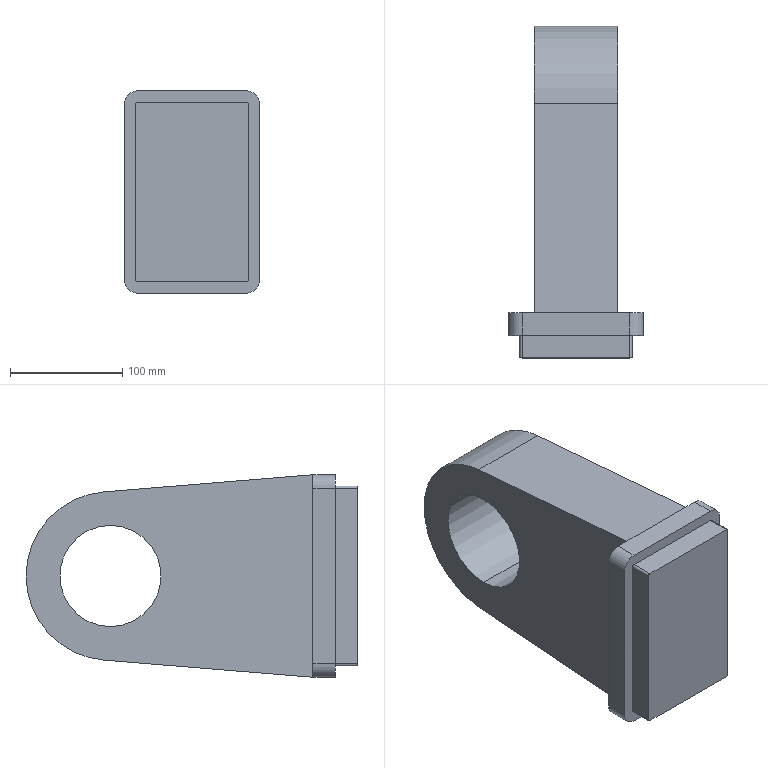Part | SolidWorks | features ICE 2, Extrusion 1 | 1 solid | 27 faces | box 120 x 295 x 180 mm | volume 3133759 mm3 | plane 16 | cylinder 11 | commonest cylinder face diameters 4 x4 24 x4 90 x2 150 x1
STEP:
#1=CARTESIAN_POINT('',(37.,200.,45.));
#2=VERTEX_POINT('',#1);
#3=CARTESIAN_POINT('',(37.,200.,-45.));
#4=VERTEX_POINT('',#3);
#5=CARTESIAN_POINT('',(37.,200.,0.));
#6=DIRECTION('',(1.,0.,0.));
#7=DIRECTION('',(0.,0.,-1.));
#8=AXIS2_PLACEMENT_3D('',#5,#6,#7);
#9=CIRCLE('',#8,45.);
#10=EDGE_CURVE('',#2,#4,#9,.T.);
#11=ORIENTED_EDGE('',*,*,#10,.T.);
#12=CARTESIAN_POINT('',(-37.,200.,-45.));
#13=VERTEX_POINT('',#12);
#14=CARTESIAN_POINT('',(37.,200.,-45.));
#15=DIRECTION('',(-1.,0.,0.));
#16=VECTOR('',#15,1000.);
#17=LINE('',#14,#16);
#18=EDGE_CURVE('',#4,#13,#17,.T.);
#19=ORIENTED_EDGE('',*,*,#18,.T.);
#20=CARTESIAN_POINT('',(-37.,200.,45.));
#21=VERTEX_POINT('',#20);
#22=CARTESIAN_POINT('',(-37.,200.,0.));
#23=DIRECTION('',(1.,0.,0.));
#24=DIRECTION('',(0.,0.,-1.));
#25=AXIS2_PLACEMENT_3D('',#22,#23,#24);
#26=CIRCLE('',#25,45.);
#27=EDGE_CURVE('',#21,#13,#26,.T.);
#28=ORIENTED_EDGE('',*,*,#27,.F.);
#29=CARTESIAN_POINT('',(37.,200.,45.));
#30=DIRECTION('',(-1.,0.,0.));
#31=VECTOR('',#30,1000.);
#32=LINE('',#29,#31);
#33=EDGE_CURVE('',#2,#21,#32,.T.);
#34=ORIENTED_EDGE('',*,*,#33,.F.);
#35=EDGE_LOOP('',(#11,#19,#28,#34));
#36=FACE_OUTER_BOUND('',#35,.T.);
#37=CARTESIAN_POINT('',(37.,200.,0.));
#38=DIRECTION('',(-1.,0.,0.));
#39=DIRECTION('',(0.,0.,1.));
#40=AXIS2_PLACEMENT_3D('',#37,#38,#39);
#41=CYLINDRICAL_SURFACE('',#40,45.);
#42=ADVANCED_FACE('',(#36),#41,.F.);
#43=CARTESIAN_POINT('',(-48.,20.,90.));
#44=VERTEX_POINT('',#43);
#45=CARTESIAN_POINT('',(-37.,20.,90.));
#46=VERTEX_POINT('',#45);
#47=CARTESIAN_POINT('',(48.,20.,90.));
#48=DIRECTION('',(1.,0.,0.));
#49=VECTOR('',#48,1000.);
#50=LINE('',#47,#49);
#51=EDGE_CURVE('',#44,#46,#50,.T.);
#52=ORIENTED_EDGE('',*,*,#51,.T.);
#53=CARTESIAN_POINT('',(-37.,20.,-90.));
#54=VERTEX_POINT('',#53);
#55=CARTESIAN_POINT('',(-37.,20.,90.));
#56=DIRECTION('',(0.,0.,-1.));
#57=VECTOR('',#56,1000.);
#58=LINE('',#55,#57);
#59=EDGE_CURVE('',#46,#54,#58,.T.);
#60=ORIENTED_EDGE('',*,*,#59,.T.);
#61=CARTESIAN_POINT('',(-48.,20.,-90.));
#62=VERTEX_POINT('',#61);
#63=CARTESIAN_POINT('',(48.,20.,-90.));
#64=DIRECTION('',(-1.,0.,0.));
#65=VECTOR('',#64,1000.);
#66=LINE('',#63,#65);
#67=EDGE_CURVE('',#54,#62,#66,.T.);
#68=ORIENTED_EDGE('',*,*,#67,.T.);
#69=CARTESIAN_POINT('',(-60.,20.,-78.));
#70=VERTEX_POINT('',#69);
#71=CARTESIAN_POINT('',(-48.,20.,-78.));
#72=DIRECTION('',(0.,1.,0.));
#73=DIRECTION('',(0.,0.,1.));
#74=AXIS2_PLACEMENT_3D('',#71,#72,#73);
#75=CIRCLE('',#74,12.);
#76=EDGE_CURVE('',#62,#70,#75,.T.);
#77=ORIENTED_EDGE('',*,*,#76,.T.);
#78=CARTESIAN_POINT('',(-60.,20.,78.));
#79=VERTEX_POINT('',#78);
#80=CARTESIAN_POINT('',(-60.,20.,-78.));
#81=DIRECTION('',(0.,0.,1.));
#82=VECTOR('',#81,1000.);
#83=LINE('',#80,#82);
#84=EDGE_CURVE('',#70,#79,#83,.T.);
#85=ORIENTED_EDGE('',*,*,#84,.T.);
#86=CARTESIAN_POINT('',(-48.,20.,78.));
#87=DIRECTION('',(0.,1.,0.));
#88=DIRECTION('',(0.,0.,-1.));
#89=AXIS2_PLACEMENT_3D('',#86,#87,#88);
#90=CIRCLE('',#89,12.);
#91=EDGE_CURVE('',#79,#44,#90,.T.);
#92=ORIENTED_EDGE('',*,*,#91,.T.);
#93=EDGE_LOOP('',(#52,#60,#68,#77,#85,#92));
#94=FACE_OUTER_BOUND('',#93,.T.);
#95=CARTESIAN_POINT('',(-48.,20.,-78.));
#96=DIRECTION('',(0.,1.,0.));
#97=DIRECTION('',(0.,0.,1.));
#98=AXIS2_PLACEMENT_3D('',#95,#96,#97);
#99=PLANE('',#98);
#100=ADVANCED_FACE('',(#94),#99,.T.);
#101=CARTESIAN_POINT('',(-48.,0.,-90.));
#102=VERTEX_POINT('',#101);
#103=CARTESIAN_POINT('',(-60.,0.,-78.));
#104=VERTEX_POINT('',#103);
#105=CARTESIAN_POINT('',(-48.,0.,-78.));
#106=DIRECTION('',(0.,1.,0.));
#107=DIRECTION('',(0.,0.,1.));
#108=AXIS2_PLACEMENT_3D('',#105,#106,#107);
#109=CIRCLE('',#108,12.);
#110=EDGE_CURVE('',#102,#104,#109,.T.);
#111=ORIENTED_EDGE('',*,*,#110,.F.);
#112=CARTESIAN_POINT('',(48.,0.,-90.));
#113=VERTEX_POINT('',#112);
#114=CARTESIAN_POINT('',(48.,0.,-90.));
#115=DIRECTION('',(-1.,0.,0.));
#116=VECTOR('',#115,1000.);
#117=LINE('',#114,#116);
#118=EDGE_CURVE('',#113,#102,#117,.T.);
#119=ORIENTED_EDGE('',*,*,#118,.F.);
#120=CARTESIAN_POINT('',(60.,0.,-78.));
#121=VERTEX_POINT('',#120);
#122=CARTESIAN_POINT('',(48.,0.,-78.));
#123=DIRECTION('',(0.,1.,0.));
#124=DIRECTION('',(0.,0.,-1.));
#125=AXIS2_PLACEMENT_3D('',#122,#123,#124);
#126=CIRCLE('',#125,12.);
#127=EDGE_CURVE('',#121,#113,#126,.T.);
#128=ORIENTED_EDGE('',*,*,#127,.F.);
#129=CARTESIAN_POINT('',(60.,0.,78.));
#130=VERTEX_POINT('',#129);
#131=CARTESIAN_POINT('',(60.,0.,-78.));
#132=DIRECTION('',(0.,0.,-1.));
#133=VECTOR('',#132,1000.);
#134=LINE('',#131,#133);
#135=EDGE_CURVE('',#130,#121,#134,.T.);
#136=ORIENTED_EDGE('',*,*,#135,.F.);
#137=CARTESIAN_POINT('',(48.,0.,90.));
#138=VERTEX_POINT('',#137);
#139=CARTESIAN_POINT('',(48.,0.,78.));
#140=DIRECTION('',(0.,1.,0.));
#141=DIRECTION('',(0.,0.,1.));
#142=AXIS2_PLACEMENT_3D('',#139,#140,#141);
#143=CIRCLE('',#142,12.);
#144=EDGE_CURVE('',#138,#130,#143,.T.);
#145=ORIENTED_EDGE('',*,*,#144,.F.);
#146=CARTESIAN_POINT('',(-48.,0.,90.));
#147=VERTEX_POINT('',#146);
#148=CARTESIAN_POINT('',(48.,0.,90.));
#149=DIRECTION('',(1.,0.,0.));
#150=VECTOR('',#149,1000.);
#151=LINE('',#148,#150);
#152=EDGE_CURVE('',#147,#138,#151,.T.);
#153=ORIENTED_EDGE('',*,*,#152,.F.);
#154=CARTESIAN_POINT('',(-60.,0.,78.));
#155=VERTEX_POINT('',#154);
#156=CARTESIAN_POINT('',(-48.,0.,78.));
#157=DIRECTION('',(0.,1.,0.));
#158=DIRECTION('',(0.,0.,-1.));
#159=AXIS2_PLACEMENT_3D('',#156,#157,#158);
#160=CIRCLE('',#159,12.);
#161=EDGE_CURVE('',#155,#147,#160,.T.);
#162=ORIENTED_EDGE('',*,*,#161,.F.);
#163=CARTESIAN_POINT('',(-60.,0.,-78.));
#164=DIRECTION('',(0.,0.,1.));
#165=VECTOR('',#164,1000.);
#166=LINE('',#163,#165);
#167=EDGE_CURVE('',#104,#155,#166,.T.);
#168=ORIENTED_EDGE('',*,*,#167,.F.);
#169=EDGE_LOOP('',(#111,#119,#128,#136,#145,#153,#162,#168));
#170=FACE_OUTER_BOUND('',#169,.T.);
#171=CARTESIAN_POINT('',(-50.,0.,-78.));
#172=VERTEX_POINT('',#171);
#173=CARTESIAN_POINT('',(-48.,0.,-80.));
#174=VERTEX_POINT('',#173);
#175=CARTESIAN_POINT('',(-48.,0.,-78.));
#176=DIRECTION('',(0.,-1.,0.));
#177=DIRECTION('',(0.,0.,-1.));
#178=AXIS2_PLACEMENT_3D('',#175,#176,#177);
#179=CIRCLE('',#178,2.);
#180=EDGE_CURVE('',#172,#174,#179,.T.);
#181=ORIENTED_EDGE('',*,*,#180,.F.);
#182=CARTESIAN_POINT('',(-50.,0.,78.));
#183=VERTEX_POINT('',#182);
#184=CARTESIAN_POINT('',(-50.,0.,78.));
#185=DIRECTION('',(0.,0.,-1.));
#186=VECTOR('',#185,1000.);
#187=LINE('',#184,#186);
#188=EDGE_CURVE('',#183,#172,#187,.T.);
#189=ORIENTED_EDGE('',*,*,#188,.F.);
#190=CARTESIAN_POINT('',(-48.,0.,80.));
#191=VERTEX_POINT('',#190);
#192=CARTESIAN_POINT('',(-48.,0.,78.));
#193=DIRECTION('',(0.,-1.,0.));
#194=DIRECTION('',(0.,0.,-1.));
#195=AXIS2_PLACEMENT_3D('',#192,#193,#194);
#196=CIRCLE('',#195,2.);
#197=EDGE_CURVE('',#191,#183,#196,.T.);
#198=ORIENTED_EDGE('',*,*,#197,.F.);
#199=CARTESIAN_POINT('',(48.,0.,80.));
#200=VERTEX_POINT('',#199);
#201=CARTESIAN_POINT('',(48.,0.,80.));
#202=DIRECTION('',(-1.,0.,0.));
#203=VECTOR('',#202,1000.);
#204=LINE('',#201,#203);
#205=EDGE_CURVE('',#200,#191,#204,.T.);
#206=ORIENTED_EDGE('',*,*,#205,.F.);
#207=CARTESIAN_POINT('',(50.,0.,78.));
#208=VERTEX_POINT('',#207);
#209=CARTESIAN_POINT('',(48.,0.,78.));
#210=DIRECTION('',(0.,-1.,0.));
#211=DIRECTION('',(0.,0.,-1.));
#212=AXIS2_PLACEMENT_3D('',#209,#210,#211);
#213=CIRCLE('',#212,2.);
#214=EDGE_CURVE('',#208,#200,#213,.T.);
#215=ORIENTED_EDGE('',*,*,#214,.F.);
#216=CARTESIAN_POINT('',(50.,0.,-78.));
#217=VERTEX_POINT('',#216);
#218=CARTESIAN_POINT('',(50.,0.,-78.));
#219=DIRECTION('',(0.,0.,1.));
#220=VECTOR('',#219,1000.);
#221=LINE('',#218,#220);
#222=EDGE_CURVE('',#217,#208,#221,.T.);
#223=ORIENTED_EDGE('',*,*,#222,.F.);
#224=CARTESIAN_POINT('',(48.,0.,-80.));
#225=VERTEX_POINT('',#224);
#226=CARTESIAN_POINT('',(48.,0.,-78.));
#227=DIRECTION('',(0.,-1.,0.));
#228=DIRECTION('',(0.,0.,-1.));
#229=AXIS2_PLACEMENT_3D('',#226,#227,#228);
#230=CIRCLE('',#229,2.);
#231=EDGE_CURVE('',#225,#217,#230,.T.);
#232=ORIENTED_EDGE('',*,*,#231,.F.);
#233=CARTESIAN_POINT('',(-48.,0.,-80.));
#234=DIRECTION('',(1.,0.,0.));
#235=VECTOR('',#234,1000.);
#236=LINE('',#233,#235);
#237=EDGE_CURVE('',#174,#225,#236,.T.);
#238=ORIENTED_EDGE('',*,*,#237,.F.);
#239=EDGE_LOOP('',(#181,#189,#198,#206,#215,#223,#232,#238));
#240=FACE_BOUND('',#239,.T.);
#241=CARTESIAN_POINT('',(-48.,0.,-78.));
#242=DIRECTION('',(0.,1.,0.));
#243=DIRECTION('',(0.,0.,1.));
#244=AXIS2_PLACEMENT_3D('',#241,#242,#243);
#245=PLANE('',#244);
#246=ADVANCED_FACE('',(#170,#240),#245,.F.);
#247=ORIENTED_EDGE('',*,*,#110,.T.);
#248=CARTESIAN_POINT('',(-60.,20.,-78.));
#249=DIRECTION('',(0.,-1.,0.));
#250=VECTOR('',#249,1000.);
#251=LINE('',#248,#250);
#252=EDGE_CURVE('',#70,#104,#251,.T.);
#253=ORIENTED_EDGE('',*,*,#252,.F.);
#254=ORIENTED_EDGE('',*,*,#76,.F.);
#255=CARTESIAN_POINT('',(-48.,20.,-90.));
#256=DIRECTION('',(0.,-1.,0.));
#257=VECTOR('',#256,1000.);
#258=LINE('',#255,#257);
#259=EDGE_CURVE('',#62,#102,#258,.T.);
#260=ORIENTED_EDGE('',*,*,#259,.T.);
#261=EDGE_LOOP('',(#247,#253,#254,#260));
#262=FACE_OUTER_BOUND('',#261,.T.);
#263=CARTESIAN_POINT('',(-48.,20.,-78.));
#264=DIRECTION('',(0.,-1.,0.));
#265=DIRECTION('',(0.,0.,-1.));
#266=AXIS2_PLACEMENT_3D('',#263,#264,#265);
#267=CYLINDRICAL_SURFACE('',#266,12.);
#268=ADVANCED_FACE('',(#262),#267,.T.);
#269=ORIENTED_EDGE('',*,*,#167,.T.);
#270=CARTESIAN_POINT('',(-60.,20.,78.));
#271=DIRECTION('',(0.,-1.,0.));
#272=VECTOR('',#271,1000.);
#273=LINE('',#270,#272);
#274=EDGE_CURVE('',#79,#155,#273,.T.);
#275=ORIENTED_EDGE('',*,*,#274,.F.);
#276=ORIENTED_EDGE('',*,*,#84,.F.);
#277=ORIENTED_EDGE('',*,*,#252,.T.);
#278=EDGE_LOOP('',(#269,#275,#276,#277));
#279=FACE_OUTER_BOUND('',#278,.T.);
#280=CARTESIAN_POINT('',(-60.,20.,-78.));
#281=DIRECTION('',(1.,0.,0.));
#282=DIRECTION('',(0.,0.,-1.));
#283=AXIS2_PLACEMENT_3D('',#280,#281,#282);
#284=PLANE('',#283);
#285=ADVANCED_FACE('',(#279),#284,.F.);
#286=ORIENTED_EDGE('',*,*,#161,.T.);
#287=CARTESIAN_POINT('',(-48.,20.,90.));
#288=DIRECTION('',(0.,-1.,0.));
#289=VECTOR('',#288,1000.);
#290=LINE('',#287,#289);
#291=EDGE_CURVE('',#44,#147,#290,.T.);
#292=ORIENTED_EDGE('',*,*,#291,.F.);
#293=ORIENTED_EDGE('',*,*,#91,.F.);
#294=ORIENTED_EDGE('',*,*,#274,.T.);
#295=EDGE_LOOP('',(#286,#292,#293,#294));
#296=FACE_OUTER_BOUND('',#295,.T.);
#297=CARTESIAN_POINT('',(-48.,20.,78.));
#298=DIRECTION('',(0.,-1.,0.));
#299=DIRECTION('',(0.,0.,-1.));
#300=AXIS2_PLACEMENT_3D('',#297,#298,#299);
#301=CYLINDRICAL_SURFACE('',#300,12.);
#302=ADVANCED_FACE('',(#296),#301,.T.);
#303=ORIENTED_EDGE('',*,*,#152,.T.);
#304=CARTESIAN_POINT('',(48.,20.,90.));
#305=VERTEX_POINT('',#304);
#306=CARTESIAN_POINT('',(48.,20.,90.));
#307=DIRECTION('',(0.,-1.,0.));
#308=VECTOR('',#307,1000.);
#309=LINE('',#306,#308);
#310=EDGE_CURVE('',#305,#138,#309,.T.);
#311=ORIENTED_EDGE('',*,*,#310,.F.);
#312=CARTESIAN_POINT('',(37.,20.,90.));
#313=VERTEX_POINT('',#312);
#314=CARTESIAN_POINT('',(48.,20.,90.));
#315=DIRECTION('',(1.,0.,0.));
#316=VECTOR('',#315,1000.);
#317=LINE('',#314,#316);
#318=EDGE_CURVE('',#313,#305,#317,.T.);
#319=ORIENTED_EDGE('',*,*,#318,.F.);
#320=CARTESIAN_POINT('',(37.,20.,90.));
#321=DIRECTION('',(-1.,0.,0.));
#322=VECTOR('',#321,1000.);
#323=LINE('',#320,#322);
#324=EDGE_CURVE('',#313,#46,#323,.T.);
#325=ORIENTED_EDGE('',*,*,#324,.T.);
#326=ORIENTED_EDGE('',*,*,#51,.F.);
#327=ORIENTED_EDGE('',*,*,#291,.T.);
#328=EDGE_LOOP('',(#303,#311,#319,#325,#326,#327));
#329=FACE_OUTER_BOUND('',#328,.T.);
#330=CARTESIAN_POINT('',(48.,20.,90.));
#331=DIRECTION('',(0.,0.,-1.));
#332=DIRECTION('',(-1.,0.,0.));
#333=AXIS2_PLACEMENT_3D('',#330,#331,#332);
#334=PLANE('',#333);
#335=ADVANCED_FACE('',(#329),#334,.F.);
#336=ORIENTED_EDGE('',*,*,#144,.T.);
#337=CARTESIAN_POINT('',(60.,20.,78.));
#338=VERTEX_POINT('',#337);
#339=CARTESIAN_POINT('',(60.,20.,78.));
#340=DIRECTION('',(0.,-1.,0.));
#341=VECTOR('',#340,1000.);
#342=LINE('',#339,#341);
#343=EDGE_CURVE('',#338,#130,#342,.T.);
#344=ORIENTED_EDGE('',*,*,#343,.F.);
#345=CARTESIAN_POINT('',(48.,20.,78.));
#346=DIRECTION('',(0.,1.,0.));
#347=DIRECTION('',(0.,0.,1.));
#348=AXIS2_PLACEMENT_3D('',#345,#346,#347);
#349=CIRCLE('',#348,12.);
#350=EDGE_CURVE('',#305,#338,#349,.T.);
#351=ORIENTED_EDGE('',*,*,#350,.F.);
#352=ORIENTED_EDGE('',*,*,#310,.T.);
#353=EDGE_LOOP('',(#336,#344,#351,#352));
#354=FACE_OUTER_BOUND('',#353,.T.);
#355=CARTESIAN_POINT('',(48.,20.,78.));
#356=DIRECTION('',(0.,-1.,0.));
#357=DIRECTION('',(0.,0.,-1.));
#358=AXIS2_PLACEMENT_3D('',#355,#356,#357);
#359=CYLINDRICAL_SURFACE('',#358,12.);
#360=ADVANCED_FACE('',(#354),#359,.T.);
#361=ORIENTED_EDGE('',*,*,#135,.T.);
#362=CARTESIAN_POINT('',(60.,20.,-78.));
#363=VERTEX_POINT('',#362);
#364=CARTESIAN_POINT('',(60.,20.,-78.));
#365=DIRECTION('',(0.,-1.,0.));
#366=VECTOR('',#365,1000.);
#367=LINE('',#364,#366);
#368=EDGE_CURVE('',#363,#121,#367,.T.);
#369=ORIENTED_EDGE('',*,*,#368,.F.);
#370=CARTESIAN_POINT('',(60.,20.,-78.));
#371=DIRECTION('',(0.,0.,-1.));
#372=VECTOR('',#371,1000.);
#373=LINE('',#370,#372);
#374=EDGE_CURVE('',#338,#363,#373,.T.);
#375=ORIENTED_EDGE('',*,*,#374,.F.);
#376=ORIENTED_EDGE('',*,*,#343,.T.);
#377=EDGE_LOOP('',(#361,#369,#375,#376));
#378=FACE_OUTER_BOUND('',#377,.T.);
#379=CARTESIAN_POINT('',(60.,20.,-78.));
#380=DIRECTION('',(-1.,0.,0.));
#381=DIRECTION('',(0.,0.,1.));
#382=AXIS2_PLACEMENT_3D('',#379,#380,#381);
#383=PLANE('',#382);
#384=ADVANCED_FACE('',(#378),#383,.F.);
#385=ORIENTED_EDGE('',*,*,#127,.T.);
#386=CARTESIAN_POINT('',(48.,20.,-90.));
#387=VERTEX_POINT('',#386);
#388=CARTESIAN_POINT('',(48.,20.,-90.));
#389=DIRECTION('',(0.,-1.,0.));
#390=VECTOR('',#389,1000.);
#391=LINE('',#388,#390);
#392=EDGE_CURVE('',#387,#113,#391,.T.);
#393=ORIENTED_EDGE('',*,*,#392,.F.);
#394=CARTESIAN_POINT('',(48.,20.,-78.));
#395=DIRECTION('',(0.,1.,0.));
#396=DIRECTION('',(0.,0.,-1.));
#397=AXIS2_PLACEMENT_3D('',#394,#395,#396);
#398=CIRCLE('',#397,12.);
#399=EDGE_CURVE('',#363,#387,#398,.T.);
#400=ORIENTED_EDGE('',*,*,#399,.F.);
#401=ORIENTED_EDGE('',*,*,#368,.T.);
#402=EDGE_LOOP('',(#385,#393,#400,#401));
#403=FACE_OUTER_BOUND('',#402,.T.);
#404=CARTESIAN_POINT('',(48.,20.,-78.));
#405=DIRECTION('',(0.,-1.,0.));
#406=DIRECTION('',(0.,0.,-1.));
#407=AXIS2_PLACEMENT_3D('',#404,#405,#406);
#408=CYLINDRICAL_SURFACE('',#407,12.);
#409=ADVANCED_FACE('',(#403),#408,.T.);
#410=ORIENTED_EDGE('',*,*,#118,.T.);
#411=ORIENTED_EDGE('',*,*,#259,.F.);
#412=ORIENTED_EDGE('',*,*,#67,.F.);
#413=CARTESIAN_POINT('',(37.,20.,-90.));
#414=VERTEX_POINT('',#413);
#415=CARTESIAN_POINT('',(37.,20.,-90.));
#416=DIRECTION('',(-1.,0.,0.));
#417=VECTOR('',#416,1000.);
#418=LINE('',#415,#417);
#419=EDGE_CURVE('',#414,#54,#418,.T.);
#420=ORIENTED_EDGE('',*,*,#419,.F.);
#421=CARTESIAN_POINT('',(48.,20.,-90.));
#422=DIRECTION('',(-1.,0.,0.));
#423=VECTOR('',#422,1000.);
#424=LINE('',#421,#423);
#425=EDGE_CURVE('',#387,#414,#424,.T.);
#426=ORIENTED_EDGE('',*,*,#425,.F.);
#427=ORIENTED_EDGE('',*,*,#392,.T.);
#428=EDGE_LOOP('',(#410,#411,#412,#420,#426,#427));
#429=FACE_OUTER_BOUND('',#428,.T.);
#430=CARTESIAN_POINT('',(48.,20.,-90.));
#431=DIRECTION('',(0.,0.,1.));
#432=DIRECTION('',(1.,0.,0.));
#433=AXIS2_PLACEMENT_3D('',#430,#431,#432);
#434=PLANE('',#433);
#435=ADVANCED_FACE('',(#429),#434,.F.);
#436=CARTESIAN_POINT('',(37.,20.,90.));
#437=DIRECTION('',(0.,0.,-1.));
#438=VECTOR('',#437,1000.);
#439=LINE('',#436,#438);
#440=EDGE_CURVE('',#313,#414,#439,.T.);
#441=ORIENTED_EDGE('',*,*,#440,.F.);
#442=ORIENTED_EDGE('',*,*,#318,.T.);
#443=ORIENTED_EDGE('',*,*,#350,.T.);
#444=ORIENTED_EDGE('',*,*,#374,.T.);
#445=ORIENTED_EDGE('',*,*,#399,.T.);
#446=ORIENTED_EDGE('',*,*,#425,.T.);
#447=EDGE_LOOP('',(#441,#442,#443,#444,#445,#446));
#448=FACE_OUTER_BOUND('',#447,.T.);
#449=CARTESIAN_POINT('',(-48.,20.,-78.));
#450=DIRECTION('',(0.,1.,0.));
#451=DIRECTION('',(0.,0.,1.));
#452=AXIS2_PLACEMENT_3D('',#449,#450,#451);
#453=PLANE('',#452);
#454=ADVANCED_FACE('',(#448),#453,.T.);
#455=ORIENTED_EDGE('',*,*,#180,.T.);
#456=CARTESIAN_POINT('',(-48.,-20.,-80.));
#457=VERTEX_POINT('',#456);
#458=CARTESIAN_POINT('',(-48.,-20.,-80.));
#459=DIRECTION('',(0.,1.,0.));
#460=VECTOR('',#459,1000.);
#461=LINE('',#458,#460);
#462=EDGE_CURVE('',#457,#174,#461,.T.);
#463=ORIENTED_EDGE('',*,*,#462,.F.);
#464=CARTESIAN_POINT('',(-50.,-20.,-78.));
#465=VERTEX_POINT('',#464);
#466=CARTESIAN_POINT('',(-48.,-20.,-78.));
#467=DIRECTION('',(0.,-1.,0.));
#468=DIRECTION('',(0.,0.,-1.));
#469=AXIS2_PLACEMENT_3D('',#466,#467,#468);
#470=CIRCLE('',#469,2.);
#471=EDGE_CURVE('',#465,#457,#470,.T.);
#472=ORIENTED_EDGE('',*,*,#471,.F.);
#473=CARTESIAN_POINT('',(-50.,-20.,-78.));
#474=DIRECTION('',(0.,1.,0.));
#475=VECTOR('',#474,1000.);
#476=LINE('',#473,#475);
#477=EDGE_CURVE('',#465,#172,#476,.T.);
#478=ORIENTED_EDGE('',*,*,#477,.T.);
#479=EDGE_LOOP('',(#455,#463,#472,#478));
#480=FACE_OUTER_BOUND('',#479,.T.);
#481=CARTESIAN_POINT('',(-48.,-20.,-78.));
#482=DIRECTION('',(0.,1.,0.));
#483=DIRECTION('',(0.,0.,1.));
#484=AXIS2_PLACEMENT_3D('',#481,#482,#483);
#485=CYLINDRICAL_SURFACE('',#484,2.);
#486=ADVANCED_FACE('',(#480),#485,.T.);
#487=ORIENTED_EDGE('',*,*,#237,.T.);
#488=CARTESIAN_POINT('',(48.,-20.,-80.));
#489=VERTEX_POINT('',#488);
#490=CARTESIAN_POINT('',(48.,-20.,-80.));
#491=DIRECTION('',(0.,1.,0.));
#492=VECTOR('',#491,1000.);
#493=LINE('',#490,#492);
#494=EDGE_CURVE('',#489,#225,#493,.T.);
#495=ORIENTED_EDGE('',*,*,#494,.F.);
#496=CARTESIAN_POINT('',(-48.,-20.,-80.));
#497=DIRECTION('',(1.,0.,0.));
#498=VECTOR('',#497,1000.);
#499=LINE('',#496,#498);
#500=EDGE_CURVE('',#457,#489,#499,.T.);
#501=ORIENTED_EDGE('',*,*,#500,.F.);
#502=ORIENTED_EDGE('',*,*,#462,.T.);
#503=EDGE_LOOP('',(#487,#495,#501,#502));
#504=FACE_OUTER_BOUND('',#503,.T.);
#505=CARTESIAN_POINT('',(-48.,-20.,-80.));
#506=DIRECTION('',(0.,0.,1.));
#507=DIRECTION('',(1.,0.,0.));
#508=AXIS2_PLACEMENT_3D('',#505,#506,#507);
#509=PLANE('',#508);
#510=ADVANCED_FACE('',(#504),#509,.F.);
#511=ORIENTED_EDGE('',*,*,#231,.T.);
#512=CARTESIAN_POINT('',(50.,-20.,-78.));
#513=VERTEX_POINT('',#512);
#514=CARTESIAN_POINT('',(50.,-20.,-78.));
#515=DIRECTION('',(0.,1.,0.));
#516=VECTOR('',#515,1000.);
#517=LINE('',#514,#516);
#518=EDGE_CURVE('',#513,#217,#517,.T.);
#519=ORIENTED_EDGE('',*,*,#518,.F.);
#520=CARTESIAN_POINT('',(48.,-20.,-78.));
#521=DIRECTION('',(0.,-1.,0.));
#522=DIRECTION('',(0.,0.,-1.));
#523=AXIS2_PLACEMENT_3D('',#520,#521,#522);
#524=CIRCLE('',#523,2.);
#525=EDGE_CURVE('',#489,#513,#524,.T.);
#526=ORIENTED_EDGE('',*,*,#525,.F.);
#527=ORIENTED_EDGE('',*,*,#494,.T.);
#528=EDGE_LOOP('',(#511,#519,#526,#527));
#529=FACE_OUTER_BOUND('',#528,.T.);
#530=CARTESIAN_POINT('',(48.,-20.,-78.));
#531=DIRECTION('',(0.,1.,0.));
#532=DIRECTION('',(0.,0.,1.));
#533=AXIS2_PLACEMENT_3D('',#530,#531,#532);
#534=CYLINDRICAL_SURFACE('',#533,2.);
#535=ADVANCED_FACE('',(#529),#534,.T.);
#536=ORIENTED_EDGE('',*,*,#222,.T.);
#537=CARTESIAN_POINT('',(50.,-20.,78.));
#538=VERTEX_POINT('',#537);
#539=CARTESIAN_POINT('',(50.,-20.,78.));
#540=DIRECTION('',(0.,1.,0.));
#541=VECTOR('',#540,1000.);
#542=LINE('',#539,#541);
#543=EDGE_CURVE('',#538,#208,#542,.T.);
#544=ORIENTED_EDGE('',*,*,#543,.F.);
#545=CARTESIAN_POINT('',(50.,-20.,-78.));
#546=DIRECTION('',(0.,0.,1.));
#547=VECTOR('',#546,1000.);
#548=LINE('',#545,#547);
#549=EDGE_CURVE('',#513,#538,#548,.T.);
#550=ORIENTED_EDGE('',*,*,#549,.F.);
#551=ORIENTED_EDGE('',*,*,#518,.T.);
#552=EDGE_LOOP('',(#536,#544,#550,#551));
#553=FACE_OUTER_BOUND('',#552,.T.);
#554=CARTESIAN_POINT('',(50.,-20.,-78.));
#555=DIRECTION('',(-1.,0.,0.));
#556=DIRECTION('',(0.,0.,1.));
#557=AXIS2_PLACEMENT_3D('',#554,#555,#556);
#558=PLANE('',#557);
#559=ADVANCED_FACE('',(#553),#558,.F.);
#560=ORIENTED_EDGE('',*,*,#214,.T.);
#561=CARTESIAN_POINT('',(48.,-20.,80.));
#562=VERTEX_POINT('',#561);
#563=CARTESIAN_POINT('',(48.,-20.,80.));
#564=DIRECTION('',(0.,1.,0.));
#565=VECTOR('',#564,1000.);
#566=LINE('',#563,#565);
#567=EDGE_CURVE('',#562,#200,#566,.T.);
#568=ORIENTED_EDGE('',*,*,#567,.F.);
#569=CARTESIAN_POINT('',(48.,-20.,78.));
#570=DIRECTION('',(0.,-1.,0.));
#571=DIRECTION('',(0.,0.,-1.));
#572=AXIS2_PLACEMENT_3D('',#569,#570,#571);
#573=CIRCLE('',#572,2.);
#574=EDGE_CURVE('',#538,#562,#573,.T.);
#575=ORIENTED_EDGE('',*,*,#574,.F.);
#576=ORIENTED_EDGE('',*,*,#543,.T.);
#577=EDGE_LOOP('',(#560,#568,#575,#576));
#578=FACE_OUTER_BOUND('',#577,.T.);
#579=CARTESIAN_POINT('',(48.,-20.,78.));
#580=DIRECTION('',(0.,1.,0.));
#581=DIRECTION('',(0.,0.,1.));
#582=AXIS2_PLACEMENT_3D('',#579,#580,#581);
#583=CYLINDRICAL_SURFACE('',#582,2.);
#584=ADVANCED_FACE('',(#578),#583,.T.);
#585=ORIENTED_EDGE('',*,*,#205,.T.);
#586=CARTESIAN_POINT('',(-48.,-20.,80.));
#587=VERTEX_POINT('',#586);
#588=CARTESIAN_POINT('',(-48.,-20.,80.));
#589=DIRECTION('',(0.,1.,0.));
#590=VECTOR('',#589,1000.);
#591=LINE('',#588,#590);
#592=EDGE_CURVE('',#587,#191,#591,.T.);
#593=ORIENTED_EDGE('',*,*,#592,.F.);
#594=CARTESIAN_POINT('',(48.,-20.,80.));
#595=DIRECTION('',(-1.,0.,0.));
#596=VECTOR('',#595,1000.);
#597=LINE('',#594,#596);
#598=EDGE_CURVE('',#562,#587,#597,.T.);
#599=ORIENTED_EDGE('',*,*,#598,.F.);
#600=ORIENTED_EDGE('',*,*,#567,.T.);
#601=EDGE_LOOP('',(#585,#593,#599,#600));
#602=FACE_OUTER_BOUND('',#601,.T.);
#603=CARTESIAN_POINT('',(48.,-20.,80.));
#604=DIRECTION('',(0.,0.,-1.));
#605=DIRECTION('',(-1.,0.,0.));
#606=AXIS2_PLACEMENT_3D('',#603,#604,#605);
#607=PLANE('',#606);
#608=ADVANCED_FACE('',(#602),#607,.F.);
#609=ORIENTED_EDGE('',*,*,#197,.T.);
#610=CARTESIAN_POINT('',(-50.,-20.,78.));
#611=VERTEX_POINT('',#610);
#612=CARTESIAN_POINT('',(-50.,-20.,78.));
#613=DIRECTION('',(0.,1.,0.));
#614=VECTOR('',#613,1000.);
#615=LINE('',#612,#614);
#616=EDGE_CURVE('',#611,#183,#615,.T.);
#617=ORIENTED_EDGE('',*,*,#616,.F.);
#618=CARTESIAN_POINT('',(-48.,-20.,78.));
#619=DIRECTION('',(0.,-1.,0.));
#620=DIRECTION('',(0.,0.,-1.));
#621=AXIS2_PLACEMENT_3D('',#618,#619,#620);
#622=CIRCLE('',#621,2.);
#623=EDGE_CURVE('',#587,#611,#622,.T.);
#624=ORIENTED_EDGE('',*,*,#623,.F.);
#625=ORIENTED_EDGE('',*,*,#592,.T.);
#626=EDGE_LOOP('',(#609,#617,#624,#625));
#627=FACE_OUTER_BOUND('',#626,.T.);
#628=CARTESIAN_POINT('',(-48.,-20.,78.));
#629=DIRECTION('',(0.,1.,0.));
#630=DIRECTION('',(0.,0.,1.));
#631=AXIS2_PLACEMENT_3D('',#628,#629,#630);
#632=CYLINDRICAL_SURFACE('',#631,2.);
#633=ADVANCED_FACE('',(#627),#632,.T.);
#634=ORIENTED_EDGE('',*,*,#188,.T.);
#635=ORIENTED_EDGE('',*,*,#477,.F.);
#636=CARTESIAN_POINT('',(-50.,-20.,78.));
#637=DIRECTION('',(0.,0.,-1.));
#638=VECTOR('',#637,1000.);
#639=LINE('',#636,#638);
#640=EDGE_CURVE('',#611,#465,#639,.T.);
#641=ORIENTED_EDGE('',*,*,#640,.F.);
#642=ORIENTED_EDGE('',*,*,#616,.T.);
#643=EDGE_LOOP('',(#634,#635,#641,#642));
#644=FACE_OUTER_BOUND('',#643,.T.);
#645=CARTESIAN_POINT('',(-50.,-20.,78.));
#646=DIRECTION('',(1.,0.,0.));
#647=DIRECTION('',(0.,0.,-1.));
#648=AXIS2_PLACEMENT_3D('',#645,#646,#647);
#649=PLANE('',#648);
#650=ADVANCED_FACE('',(#644),#649,.F.);
#651=ORIENTED_EDGE('',*,*,#471,.T.);
#652=ORIENTED_EDGE('',*,*,#500,.T.);
#653=ORIENTED_EDGE('',*,*,#525,.T.);
#654=ORIENTED_EDGE('',*,*,#549,.T.);
#655=ORIENTED_EDGE('',*,*,#574,.T.);
#656=ORIENTED_EDGE('',*,*,#598,.T.);
#657=ORIENTED_EDGE('',*,*,#623,.T.);
#658=ORIENTED_EDGE('',*,*,#640,.T.);
#659=EDGE_LOOP('',(#651,#652,#653,#654,#655,#656,#657,#658));
#660=FACE_OUTER_BOUND('',#659,.T.);
#661=CARTESIAN_POINT('',(-48.,-20.,-78.));
#662=DIRECTION('',(0.,-1.,0.));
#663=DIRECTION('',(0.,0.,-1.));
#664=AXIS2_PLACEMENT_3D('',#661,#662,#663);
#665=PLANE('',#664);
#666=ADVANCED_FACE('',(#660),#665,.T.);
#667=CARTESIAN_POINT('',(37.,206.125,-74.749));
#668=VERTEX_POINT('',#667);
#669=CARTESIAN_POINT('',(37.,206.125,74.749));
#670=VERTEX_POINT('',#669);
#671=CARTESIAN_POINT('',(37.,200.,0.));
#672=DIRECTION('',(1.,0.,0.));
#673=DIRECTION('',(0.,0.,-1.));
#674=AXIS2_PLACEMENT_3D('',#671,#672,#673);
#675=CIRCLE('',#674,75.);
#676=EDGE_CURVE('',#668,#670,#675,.T.);
#677=ORIENTED_EDGE('',*,*,#676,.T.);
#678=CARTESIAN_POINT('',(37.,206.125,74.749));
#679=DIRECTION('',(0.,-0.9967,0.08166));
#680=VECTOR('',#679,1000.);
#681=LINE('',#678,#680);
#682=EDGE_CURVE('',#670,#313,#681,.T.);
#683=ORIENTED_EDGE('',*,*,#682,.T.);
#684=ORIENTED_EDGE('',*,*,#440,.T.);
#685=CARTESIAN_POINT('',(37.,206.125,-74.749));
#686=DIRECTION('',(0.,0.9967,0.08166));
#687=VECTOR('',#686,1000.);
#688=LINE('',#685,#687);
#689=EDGE_CURVE('',#414,#668,#688,.T.);
#690=ORIENTED_EDGE('',*,*,#689,.T.);
#691=EDGE_LOOP('',(#677,#683,#684,#690));
#692=FACE_OUTER_BOUND('',#691,.T.);
#693=ORIENTED_EDGE('',*,*,#10,.F.);
#694=CARTESIAN_POINT('',(37.,200.,0.));
#695=DIRECTION('',(1.,0.,0.));
#696=DIRECTION('',(0.,0.,-1.));
#697=AXIS2_PLACEMENT_3D('',#694,#695,#696);
#698=CIRCLE('',#697,45.);
#699=EDGE_CURVE('',#4,#2,#698,.T.);
#700=ORIENTED_EDGE('',*,*,#699,.F.);
#701=EDGE_LOOP('',(#693,#700));
#702=FACE_BOUND('',#701,.T.);
#703=CARTESIAN_POINT('',(37.,200.,0.));
#704=DIRECTION('',(1.,0.,0.));
#705=DIRECTION('',(0.,0.,-1.));
#706=AXIS2_PLACEMENT_3D('',#703,#704,#705);
#707=PLANE('',#706);
#708=ADVANCED_FACE('',(#692,#702),#707,.T.);
#709=CARTESIAN_POINT('',(-37.,206.125,-74.749));
#710=VERTEX_POINT('',#709);
#711=CARTESIAN_POINT('',(-37.,206.125,74.749));
#712=VERTEX_POINT('',#711);
#713=CARTESIAN_POINT('',(-37.,200.,0.));
#714=DIRECTION('',(1.,0.,0.));
#715=DIRECTION('',(0.,0.,-1.));
#716=AXIS2_PLACEMENT_3D('',#713,#714,#715);
#717=CIRCLE('',#716,75.);
#718=EDGE_CURVE('',#710,#712,#717,.T.);
#719=ORIENTED_EDGE('',*,*,#718,.F.);
#720=CARTESIAN_POINT('',(-37.,206.125,-74.749));
#721=DIRECTION('',(0.,0.9967,0.08166));
#722=VECTOR('',#721,1000.);
#723=LINE('',#720,#722);
#724=EDGE_CURVE('',#54,#710,#723,.T.);
#725=ORIENTED_EDGE('',*,*,#724,.F.);
#726=ORIENTED_EDGE('',*,*,#59,.F.);
#727=CARTESIAN_POINT('',(-37.,206.125,74.749));
#728=DIRECTION('',(0.,-0.9967,0.08166));
#729=VECTOR('',#728,1000.);
#730=LINE('',#727,#729);
#731=EDGE_CURVE('',#712,#46,#730,.T.);
#732=ORIENTED_EDGE('',*,*,#731,.F.);
#733=EDGE_LOOP('',(#719,#725,#726,#732));
#734=FACE_OUTER_BOUND('',#733,.T.);
#735=ORIENTED_EDGE('',*,*,#27,.T.);
#736=CARTESIAN_POINT('',(-37.,200.,0.));
#737=DIRECTION('',(1.,0.,0.));
#738=DIRECTION('',(0.,0.,-1.));
#739=AXIS2_PLACEMENT_3D('',#736,#737,#738);
#740=CIRCLE('',#739,45.);
#741=EDGE_CURVE('',#13,#21,#740,.T.);
#742=ORIENTED_EDGE('',*,*,#741,.T.);
#743=EDGE_LOOP('',(#735,#742));
#744=FACE_BOUND('',#743,.T.);
#745=CARTESIAN_POINT('',(-37.,200.,0.));
#746=DIRECTION('',(1.,0.,0.));
#747=DIRECTION('',(0.,0.,-1.));
#748=AXIS2_PLACEMENT_3D('',#745,#746,#747);
#749=PLANE('',#748);
#750=ADVANCED_FACE('',(#734,#744),#749,.F.);
#751=ORIENTED_EDGE('',*,*,#718,.T.);
#752=CARTESIAN_POINT('',(37.,206.125,74.749));
#753=DIRECTION('',(-1.,0.,0.));
#754=VECTOR('',#753,1000.);
#755=LINE('',#752,#754);
#756=EDGE_CURVE('',#670,#712,#755,.T.);
#757=ORIENTED_EDGE('',*,*,#756,.F.);
#758=ORIENTED_EDGE('',*,*,#676,.F.);
#759=CARTESIAN_POINT('',(37.,206.125,-74.749));
#760=DIRECTION('',(-1.,0.,0.));
#761=VECTOR('',#760,1000.);
#762=LINE('',#759,#761);
#763=EDGE_CURVE('',#668,#710,#762,.T.);
#764=ORIENTED_EDGE('',*,*,#763,.T.);
#765=EDGE_LOOP('',(#751,#757,#758,#764));
#766=FACE_OUTER_BOUND('',#765,.T.);
#767=CARTESIAN_POINT('',(37.,200.,0.));
#768=DIRECTION('',(-1.,0.,0.));
#769=DIRECTION('',(0.,0.,1.));
#770=AXIS2_PLACEMENT_3D('',#767,#768,#769);
#771=CYLINDRICAL_SURFACE('',#770,75.);
#772=ADVANCED_FACE('',(#766),#771,.T.);
#773=ORIENTED_EDGE('',*,*,#731,.T.);
#774=ORIENTED_EDGE('',*,*,#324,.F.);
#775=ORIENTED_EDGE('',*,*,#682,.F.);
#776=ORIENTED_EDGE('',*,*,#756,.T.);
#777=EDGE_LOOP('',(#773,#774,#775,#776));
#778=FACE_OUTER_BOUND('',#777,.T.);
#779=CARTESIAN_POINT('',(37.,206.125,74.749));
#780=DIRECTION('',(0.,-0.08166,-0.9967));
#781=DIRECTION('',(0.,0.9967,-0.08166));
#782=AXIS2_PLACEMENT_3D('',#779,#780,#781);
#783=PLANE('',#782);
#784=ADVANCED_FACE('',(#778),#783,.F.);
#785=ORIENTED_EDGE('',*,*,#724,.T.);
#786=ORIENTED_EDGE('',*,*,#763,.F.);
#787=ORIENTED_EDGE('',*,*,#689,.F.);
#788=ORIENTED_EDGE('',*,*,#419,.T.);
#789=EDGE_LOOP('',(#785,#786,#787,#788));
#790=FACE_OUTER_BOUND('',#789,.T.);
#791=CARTESIAN_POINT('',(37.,206.125,-74.749));
#792=DIRECTION('',(0.,-0.08166,0.9967));
#793=DIRECTION('',(0.,-0.9967,-0.08166));
#794=AXIS2_PLACEMENT_3D('',#791,#792,#793);
#795=PLANE('',#794);
#796=ADVANCED_FACE('',(#790),#795,.F.);
#797=ORIENTED_EDGE('',*,*,#18,.F.);
#798=ORIENTED_EDGE('',*,*,#699,.T.);
#799=ORIENTED_EDGE('',*,*,#33,.T.);
#800=ORIENTED_EDGE('',*,*,#741,.F.);
#801=EDGE_LOOP('',(#797,#798,#799,#800));
#802=FACE_OUTER_BOUND('',#801,.T.);
#803=CARTESIAN_POINT('',(37.,200.,0.));
#804=DIRECTION('',(-1.,0.,0.));
#805=DIRECTION('',(0.,0.,1.));
#806=AXIS2_PLACEMENT_3D('',#803,#804,#805);
#807=CYLINDRICAL_SURFACE('',#806,45.);
#808=ADVANCED_FACE('',(#802),#807,.F.);
#809=CLOSED_SHELL('',(#42,#100,#246,#268,#285,#302,#335,#360,#384,#409,#435,#454,#486,#510,#535,#559,#584,#608,#633,#650,#666,#708,#750,#772,#784,#796,#808));
#810=MANIFOLD_SOLID_BREP('',#809);
#811=CARTESIAN_POINT('',(0.,0.,0.));
#812=DIRECTION('',(0.,0.,1.));
#813=DIRECTION('',(1.,0.,0.));
#814=AXIS2_PLACEMENT_3D('',#811,#812,#813);
#815=(LENGTH_UNIT()NAMED_UNIT(*)SI_UNIT(.MILLI.,.METRE.));
#816=UNCERTAINTY_MEASURE_WITH_UNIT(LENGTH_MEASURE(0.00001),#815,'','');
#817=(NAMED_UNIT(*)PLANE_ANGLE_UNIT()SI_UNIT($,.RADIAN.));
#818=(NAMED_UNIT(*)SI_UNIT($,.STERADIAN.)SOLID_ANGLE_UNIT());
#819=(GEOMETRIC_REPRESENTATION_CONTEXT(3)GLOBAL_UNCERTAINTY_ASSIGNED_CONTEXT((#816))GLOBAL_UNIT_ASSIGNED_CONTEXT((#815,#817,#818))REPRESENTATION_CONTEXT('',''));
#820=ADVANCED_BREP_SHAPE_REPRESENTATION('',(#810,#814),#819);